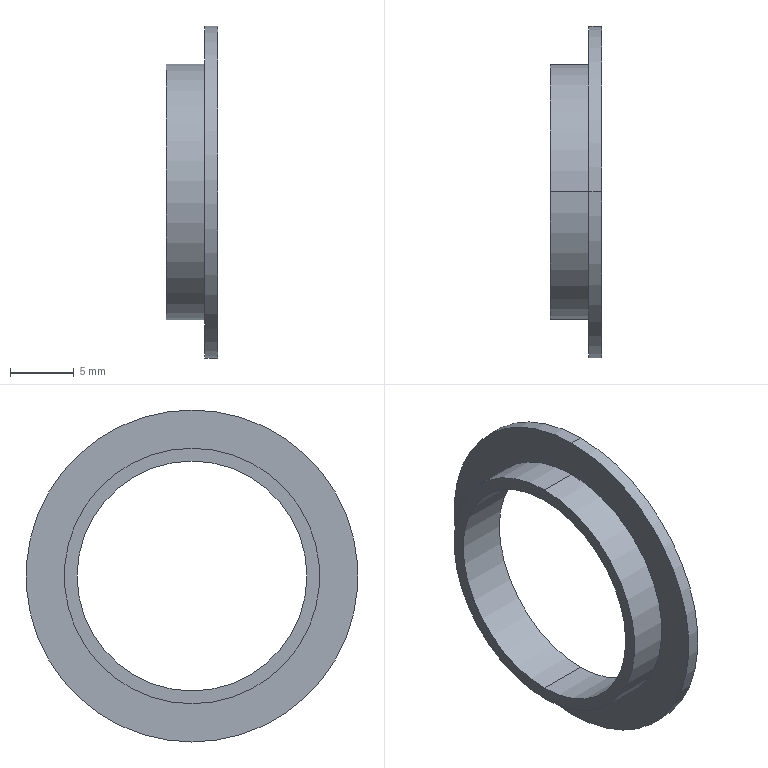Part | SolidWorks | features Revolution 1 | 1 solid | 9 faces | box 4 x 26 x 26 mm | volume 455.531 mm3 | cylinder 6 | plane 3 | commonest cylinder face diameters 18 x2 20 x2 26 x2
STEP:
#1=CARTESIAN_POINT('',(4.,0.,13.));
#2=VERTEX_POINT('',#1);
#3=CARTESIAN_POINT('',(4.,0.,-13.));
#4=VERTEX_POINT('',#3);
#5=CARTESIAN_POINT('',(4.,0.,0.));
#6=DIRECTION('',(-1.,0.,0.));
#7=DIRECTION('',(0.,0.,1.));
#8=AXIS2_PLACEMENT_3D('',#5,#6,#7);
#9=CIRCLE('',#8,13.);
#10=EDGE_CURVE('',#2,#4,#9,.T.);
#11=ORIENTED_EDGE('',*,*,#10,.T.);
#12=CARTESIAN_POINT('',(3.,0.,-13.));
#13=VERTEX_POINT('',#12);
#14=CARTESIAN_POINT('',(-397.809,0.,-13.));
#15=DIRECTION('',(-1.,0.,0.));
#16=VECTOR('',#15,1000.);
#17=LINE('',#14,#16);
#18=EDGE_CURVE('',#4,#13,#17,.T.);
#19=ORIENTED_EDGE('',*,*,#18,.T.);
#20=CARTESIAN_POINT('',(3.,0.,13.));
#21=VERTEX_POINT('',#20);
#22=CARTESIAN_POINT('',(3.,0.,0.));
#23=DIRECTION('',(-1.,0.,0.));
#24=DIRECTION('',(0.,0.,1.));
#25=AXIS2_PLACEMENT_3D('',#22,#23,#24);
#26=CIRCLE('',#25,13.);
#27=EDGE_CURVE('',#21,#13,#26,.T.);
#28=ORIENTED_EDGE('',*,*,#27,.F.);
#29=CARTESIAN_POINT('',(-397.809,0.,13.));
#30=DIRECTION('',(-1.,0.,0.));
#31=VECTOR('',#30,1000.);
#32=LINE('',#29,#31);
#33=EDGE_CURVE('',#2,#21,#32,.T.);
#34=ORIENTED_EDGE('',*,*,#33,.F.);
#35=EDGE_LOOP('',(#11,#19,#28,#34));
#36=FACE_OUTER_BOUND('',#35,.T.);
#37=CARTESIAN_POINT('',(-397.809,0.,0.));
#38=DIRECTION('',(-1.,0.,0.));
#39=DIRECTION('',(0.,0.,1.));
#40=AXIS2_PLACEMENT_3D('',#37,#38,#39);
#41=CYLINDRICAL_SURFACE('',#40,13.);
#42=ADVANCED_FACE('',(#36),#41,.T.);
#43=CARTESIAN_POINT('',(3.,0.,10.));
#44=VERTEX_POINT('',#43);
#45=CARTESIAN_POINT('',(3.,0.,-10.));
#46=VERTEX_POINT('',#45);
#47=CARTESIAN_POINT('',(3.,0.,0.));
#48=DIRECTION('',(-1.,0.,0.));
#49=DIRECTION('',(0.,0.,1.));
#50=AXIS2_PLACEMENT_3D('',#47,#48,#49);
#51=CIRCLE('',#50,10.);
#52=EDGE_CURVE('',#44,#46,#51,.T.);
#53=ORIENTED_EDGE('',*,*,#52,.T.);
#54=CARTESIAN_POINT('',(0.,0.,-10.));
#55=VERTEX_POINT('',#54);
#56=CARTESIAN_POINT('',(-397.809,0.,-10.));
#57=DIRECTION('',(-1.,0.,0.));
#58=VECTOR('',#57,1000.);
#59=LINE('',#56,#58);
#60=EDGE_CURVE('',#46,#55,#59,.T.);
#61=ORIENTED_EDGE('',*,*,#60,.T.);
#62=CARTESIAN_POINT('',(0.,0.,10.));
#63=VERTEX_POINT('',#62);
#64=CARTESIAN_POINT('',(0.,0.,0.));
#65=DIRECTION('',(-1.,0.,0.));
#66=DIRECTION('',(0.,0.,1.));
#67=AXIS2_PLACEMENT_3D('',#64,#65,#66);
#68=CIRCLE('',#67,10.);
#69=EDGE_CURVE('',#63,#55,#68,.T.);
#70=ORIENTED_EDGE('',*,*,#69,.F.);
#71=CARTESIAN_POINT('',(-397.809,0.,10.));
#72=DIRECTION('',(-1.,0.,0.));
#73=VECTOR('',#72,1000.);
#74=LINE('',#71,#73);
#75=EDGE_CURVE('',#44,#63,#74,.T.);
#76=ORIENTED_EDGE('',*,*,#75,.F.);
#77=EDGE_LOOP('',(#53,#61,#70,#76));
#78=FACE_OUTER_BOUND('',#77,.T.);
#79=CARTESIAN_POINT('',(-397.809,0.,0.));
#80=DIRECTION('',(-1.,0.,0.));
#81=DIRECTION('',(0.,0.,1.));
#82=AXIS2_PLACEMENT_3D('',#79,#80,#81);
#83=CYLINDRICAL_SURFACE('',#82,10.);
#84=ADVANCED_FACE('',(#78),#83,.T.);
#85=CARTESIAN_POINT('',(4.,0.,-9.));
#86=VERTEX_POINT('',#85);
#87=CARTESIAN_POINT('',(4.,0.,9.));
#88=VERTEX_POINT('',#87);
#89=CARTESIAN_POINT('',(4.,0.,0.));
#90=DIRECTION('',(-1.,0.,0.));
#91=DIRECTION('',(0.,0.,1.));
#92=AXIS2_PLACEMENT_3D('',#89,#90,#91);
#93=CIRCLE('',#92,9.);
#94=EDGE_CURVE('',#86,#88,#93,.T.);
#95=ORIENTED_EDGE('',*,*,#94,.F.);
#96=CARTESIAN_POINT('',(0.,0.,-9.));
#97=VERTEX_POINT('',#96);
#98=CARTESIAN_POINT('',(-397.809,0.,-9.));
#99=DIRECTION('',(-1.,0.,0.));
#100=VECTOR('',#99,1000.);
#101=LINE('',#98,#100);
#102=EDGE_CURVE('',#86,#97,#101,.T.);
#103=ORIENTED_EDGE('',*,*,#102,.T.);
#104=CARTESIAN_POINT('',(0.,0.,9.));
#105=VERTEX_POINT('',#104);
#106=CARTESIAN_POINT('',(0.,0.,0.));
#107=DIRECTION('',(-1.,0.,0.));
#108=DIRECTION('',(0.,0.,1.));
#109=AXIS2_PLACEMENT_3D('',#106,#107,#108);
#110=CIRCLE('',#109,9.);
#111=EDGE_CURVE('',#97,#105,#110,.T.);
#112=ORIENTED_EDGE('',*,*,#111,.T.);
#113=CARTESIAN_POINT('',(-397.809,0.,9.));
#114=DIRECTION('',(-1.,0.,0.));
#115=VECTOR('',#114,1000.);
#116=LINE('',#113,#115);
#117=EDGE_CURVE('',#88,#105,#116,.T.);
#118=ORIENTED_EDGE('',*,*,#117,.F.);
#119=EDGE_LOOP('',(#95,#103,#112,#118));
#120=FACE_OUTER_BOUND('',#119,.T.);
#121=CARTESIAN_POINT('',(-397.809,0.,0.));
#122=DIRECTION('',(-1.,0.,0.));
#123=DIRECTION('',(0.,0.,1.));
#124=AXIS2_PLACEMENT_3D('',#121,#122,#123);
#125=CYLINDRICAL_SURFACE('',#124,9.);
#126=ADVANCED_FACE('',(#120),#125,.F.);
#127=ORIENTED_EDGE('',*,*,#102,.F.);
#128=CARTESIAN_POINT('',(4.,0.,0.));
#129=DIRECTION('',(-1.,0.,0.));
#130=DIRECTION('',(0.,0.,1.));
#131=AXIS2_PLACEMENT_3D('',#128,#129,#130);
#132=CIRCLE('',#131,9.);
#133=EDGE_CURVE('',#88,#86,#132,.T.);
#134=ORIENTED_EDGE('',*,*,#133,.F.);
#135=ORIENTED_EDGE('',*,*,#117,.T.);
#136=CARTESIAN_POINT('',(0.,0.,0.));
#137=DIRECTION('',(-1.,0.,0.));
#138=DIRECTION('',(0.,0.,1.));
#139=AXIS2_PLACEMENT_3D('',#136,#137,#138);
#140=CIRCLE('',#139,9.);
#141=EDGE_CURVE('',#105,#97,#140,.T.);
#142=ORIENTED_EDGE('',*,*,#141,.T.);
#143=EDGE_LOOP('',(#127,#134,#135,#142));
#144=FACE_OUTER_BOUND('',#143,.T.);
#145=CARTESIAN_POINT('',(-397.809,0.,0.));
#146=DIRECTION('',(-1.,0.,0.));
#147=DIRECTION('',(0.,0.,1.));
#148=AXIS2_PLACEMENT_3D('',#145,#146,#147);
#149=CYLINDRICAL_SURFACE('',#148,9.);
#150=ADVANCED_FACE('',(#144),#149,.F.);
#151=ORIENTED_EDGE('',*,*,#141,.F.);
#152=ORIENTED_EDGE('',*,*,#111,.F.);
#153=EDGE_LOOP('',(#151,#152));
#154=FACE_BOUND('',#153,.T.);
#155=ORIENTED_EDGE('',*,*,#69,.T.);
#156=CARTESIAN_POINT('',(0.,0.,0.));
#157=DIRECTION('',(-1.,0.,0.));
#158=DIRECTION('',(0.,0.,1.));
#159=AXIS2_PLACEMENT_3D('',#156,#157,#158);
#160=CIRCLE('',#159,10.);
#161=EDGE_CURVE('',#55,#63,#160,.T.);
#162=ORIENTED_EDGE('',*,*,#161,.T.);
#163=EDGE_LOOP('',(#155,#162));
#164=FACE_OUTER_BOUND('',#163,.T.);
#165=CARTESIAN_POINT('',(0.,0.,-9.));
#166=DIRECTION('',(1.,0.,0.));
#167=DIRECTION('',(0.,0.,-1.));
#168=AXIS2_PLACEMENT_3D('',#165,#166,#167);
#169=PLANE('',#168);
#170=ADVANCED_FACE('',(#154,#164),#169,.F.);
#171=ORIENTED_EDGE('',*,*,#60,.F.);
#172=CARTESIAN_POINT('',(3.,0.,0.));
#173=DIRECTION('',(-1.,0.,0.));
#174=DIRECTION('',(0.,0.,1.));
#175=AXIS2_PLACEMENT_3D('',#172,#173,#174);
#176=CIRCLE('',#175,10.);
#177=EDGE_CURVE('',#46,#44,#176,.T.);
#178=ORIENTED_EDGE('',*,*,#177,.T.);
#179=ORIENTED_EDGE('',*,*,#75,.T.);
#180=ORIENTED_EDGE('',*,*,#161,.F.);
#181=EDGE_LOOP('',(#171,#178,#179,#180));
#182=FACE_OUTER_BOUND('',#181,.T.);
#183=CARTESIAN_POINT('',(-397.809,0.,0.));
#184=DIRECTION('',(-1.,0.,0.));
#185=DIRECTION('',(0.,0.,1.));
#186=AXIS2_PLACEMENT_3D('',#183,#184,#185);
#187=CYLINDRICAL_SURFACE('',#186,10.);
#188=ADVANCED_FACE('',(#182),#187,.T.);
#189=ORIENTED_EDGE('',*,*,#52,.F.);
#190=ORIENTED_EDGE('',*,*,#177,.F.);
#191=EDGE_LOOP('',(#189,#190));
#192=FACE_BOUND('',#191,.T.);
#193=ORIENTED_EDGE('',*,*,#27,.T.);
#194=CARTESIAN_POINT('',(3.,0.,0.));
#195=DIRECTION('',(-1.,0.,0.));
#196=DIRECTION('',(0.,0.,1.));
#197=AXIS2_PLACEMENT_3D('',#194,#195,#196);
#198=CIRCLE('',#197,13.);
#199=EDGE_CURVE('',#13,#21,#198,.T.);
#200=ORIENTED_EDGE('',*,*,#199,.T.);
#201=EDGE_LOOP('',(#193,#200));
#202=FACE_OUTER_BOUND('',#201,.T.);
#203=CARTESIAN_POINT('',(3.,0.,-10.));
#204=DIRECTION('',(1.,0.,0.));
#205=DIRECTION('',(0.,0.,-1.));
#206=AXIS2_PLACEMENT_3D('',#203,#204,#205);
#207=PLANE('',#206);
#208=ADVANCED_FACE('',(#192,#202),#207,.F.);
#209=ORIENTED_EDGE('',*,*,#18,.F.);
#210=CARTESIAN_POINT('',(4.,0.,0.));
#211=DIRECTION('',(-1.,0.,0.));
#212=DIRECTION('',(0.,0.,1.));
#213=AXIS2_PLACEMENT_3D('',#210,#211,#212);
#214=CIRCLE('',#213,13.);
#215=EDGE_CURVE('',#4,#2,#214,.T.);
#216=ORIENTED_EDGE('',*,*,#215,.T.);
#217=ORIENTED_EDGE('',*,*,#33,.T.);
#218=ORIENTED_EDGE('',*,*,#199,.F.);
#219=EDGE_LOOP('',(#209,#216,#217,#218));
#220=FACE_OUTER_BOUND('',#219,.T.);
#221=CARTESIAN_POINT('',(-397.809,0.,0.));
#222=DIRECTION('',(-1.,0.,0.));
#223=DIRECTION('',(0.,0.,1.));
#224=AXIS2_PLACEMENT_3D('',#221,#222,#223);
#225=CYLINDRICAL_SURFACE('',#224,13.);
#226=ADVANCED_FACE('',(#220),#225,.T.);
#227=ORIENTED_EDGE('',*,*,#10,.F.);
#228=ORIENTED_EDGE('',*,*,#215,.F.);
#229=EDGE_LOOP('',(#227,#228));
#230=FACE_OUTER_BOUND('',#229,.T.);
#231=ORIENTED_EDGE('',*,*,#133,.T.);
#232=ORIENTED_EDGE('',*,*,#94,.T.);
#233=EDGE_LOOP('',(#231,#232));
#234=FACE_BOUND('',#233,.T.);
#235=CARTESIAN_POINT('',(4.,0.,-13.));
#236=DIRECTION('',(-1.,0.,0.));
#237=DIRECTION('',(0.,0.,1.));
#238=AXIS2_PLACEMENT_3D('',#235,#236,#237);
#239=PLANE('',#238);
#240=ADVANCED_FACE('',(#230,#234),#239,.F.);
#241=CLOSED_SHELL('',(#42,#84,#126,#150,#170,#188,#208,#226,#240));
#242=MANIFOLD_SOLID_BREP('',#241);
#243=CARTESIAN_POINT('',(0.,0.,0.));
#244=DIRECTION('',(0.,0.,1.));
#245=DIRECTION('',(1.,0.,0.));
#246=AXIS2_PLACEMENT_3D('',#243,#244,#245);
#247=(LENGTH_UNIT()NAMED_UNIT(*)SI_UNIT(.MILLI.,.METRE.));
#248=UNCERTAINTY_MEASURE_WITH_UNIT(LENGTH_MEASURE(0.00001),#247,'','');
#249=(NAMED_UNIT(*)PLANE_ANGLE_UNIT()SI_UNIT($,.RADIAN.));
#250=(NAMED_UNIT(*)SI_UNIT($,.STERADIAN.)SOLID_ANGLE_UNIT());
#251=(GEOMETRIC_REPRESENTATION_CONTEXT(3)GLOBAL_UNCERTAINTY_ASSIGNED_CONTEXT((#248))GLOBAL_UNIT_ASSIGNED_CONTEXT((#247,#249,#250))REPRESENTATION_CONTEXT('',''));
#252=ADVANCED_BREP_SHAPE_REPRESENTATION('',(#242,#246),#251);